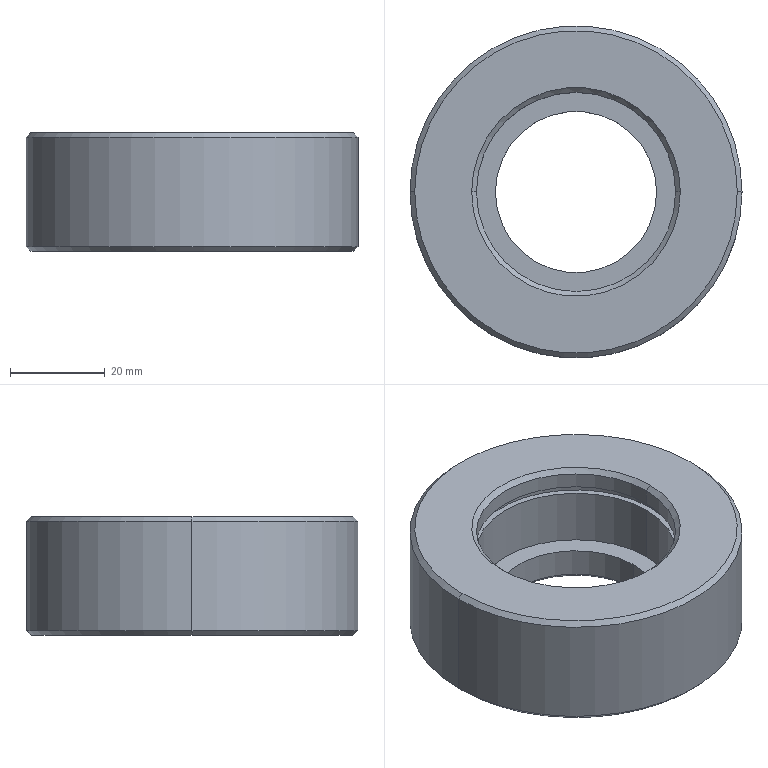Part | STEP file | 1 solid | 23 faces | box 70 x 70 x 25 mm | volume 64290 mm3 | cylinder 10 | cone 8 | plane 5 | commonest cylinder face diameters 42 x4 34 x2 44.5 x2 70 x2
STEP:
#1=CARTESIAN_POINT('',(0.,0.,0.));
#2=DIRECTION('',(0.,0.,1.));
#3=DIRECTION('',(1.,0.,0.));
#4=AXIS2_PLACEMENT_3D('',#1,#2,#3);
#5=CARTESIAN_POINT('',(21.,0.,20.7));
#6=VERTEX_POINT('',#5);
#7=CARTESIAN_POINT('',(-21.,0.,20.7));
#8=VERTEX_POINT('',#7);
#9=CARTESIAN_POINT('',(0.,0.,20.7));
#10=DIRECTION('',(0.,0.,1.));
#11=DIRECTION('',(1.,0.,0.));
#12=AXIS2_PLACEMENT_3D('',#9,#10,#11);
#13=CIRCLE('',#12,21.);
#14=CARTESIAN_POINT('',(0.,0.,20.7));
#15=DIRECTION('',(0.,0.,1.));
#16=DIRECTION('',(1.,0.,0.));
#17=AXIS2_PLACEMENT_3D('',#14,#15,#16);
#18=PLANE('',#17);
#19=CARTESIAN_POINT('',(0.,0.));
#20=DIRECTION('',(1.,0.));
#21=AXIS2_PLACEMENT_2D('',#19,#20);
#22=CIRCLE('',#21,21.);
#23=(GEOMETRIC_REPRESENTATION_CONTEXT(2)PARAMETRIC_REPRESENTATION_CONTEXT()REPRESENTATION_CONTEXT('',''));
#24=DEFINITIONAL_REPRESENTATION('',(#22),#23);
#25=PCURVE('',#18,#24);
#26=CARTESIAN_POINT('',(0.,0.,7.));
#27=DIRECTION('',(0.,0.,1.));
#28=DIRECTION('',(1.,0.,0.));
#29=AXIS2_PLACEMENT_3D('',#26,#27,#28);
#30=CYLINDRICAL_SURFACE('',#29,21.);
#31=CARTESIAN_POINT('',(0.,13.7));
#32=DIRECTION('',(1.,0.));
#33=VECTOR('',#32,1.);
#34=LINE('',#31,#33);
#35=(GEOMETRIC_REPRESENTATION_CONTEXT(2)PARAMETRIC_REPRESENTATION_CONTEXT()REPRESENTATION_CONTEXT('',''));
#36=DEFINITIONAL_REPRESENTATION('',(#34),#35);
#37=PCURVE('',#30,#36);
#38=SURFACE_CURVE('',#13,(#25,#37),.PCURVE_S1.);
#39=EDGE_CURVE('',#6,#8,#38,.T.);
#40=ORIENTED_EDGE('',*,*,#39,.T.);
#41=CARTESIAN_POINT('',(0.,0.,20.7));
#42=DIRECTION('',(0.,0.,1.));
#43=DIRECTION('',(1.,0.,0.));
#44=AXIS2_PLACEMENT_3D('',#41,#42,#43);
#45=CIRCLE('',#44,21.);
#46=CARTESIAN_POINT('',(0.,0.));
#47=DIRECTION('',(1.,0.));
#48=AXIS2_PLACEMENT_2D('',#46,#47);
#49=CIRCLE('',#48,21.);
#50=(GEOMETRIC_REPRESENTATION_CONTEXT(2)PARAMETRIC_REPRESENTATION_CONTEXT()REPRESENTATION_CONTEXT('',''));
#51=DEFINITIONAL_REPRESENTATION('',(#49),#50);
#52=PCURVE('',#18,#51);
#53=CARTESIAN_POINT('',(0.,0.,7.));
#54=DIRECTION('',(0.,0.,1.));
#55=DIRECTION('',(1.,0.,0.));
#56=AXIS2_PLACEMENT_3D('',#53,#54,#55);
#57=CYLINDRICAL_SURFACE('',#56,21.);
#58=CARTESIAN_POINT('',(0.,13.7));
#59=DIRECTION('',(1.,0.));
#60=VECTOR('',#59,1.);
#61=LINE('',#58,#60);
#62=(GEOMETRIC_REPRESENTATION_CONTEXT(2)PARAMETRIC_REPRESENTATION_CONTEXT()REPRESENTATION_CONTEXT('',''));
#63=DEFINITIONAL_REPRESENTATION('',(#61),#62);
#64=PCURVE('',#57,#63);
#65=SURFACE_CURVE('',#45,(#52,#64),.PCURVE_S1.);
#66=EDGE_CURVE('',#8,#6,#65,.T.);
#67=ORIENTED_EDGE('',*,*,#66,.T.);
#68=EDGE_LOOP('',(#40,#67));
#69=FACE_BOUND('',#68,.T.);
#70=CARTESIAN_POINT('',(-22.25,0.,20.7));
#71=VERTEX_POINT('',#70);
#72=CARTESIAN_POINT('',(22.25,0.,20.7));
#73=VERTEX_POINT('',#72);
#74=CARTESIAN_POINT('',(0.,0.,20.7));
#75=DIRECTION('',(0.,0.,-1.));
#76=DIRECTION('',(-1.,0.,0.));
#77=AXIS2_PLACEMENT_3D('',#74,#75,#76);
#78=CIRCLE('',#77,22.25);
#79=CARTESIAN_POINT('',(-22.25,0.));
#80=CARTESIAN_POINT('',(-22.25,38.538));
#81=CARTESIAN_POINT('',(11.125,19.269));
#82=CARTESIAN_POINT('',(44.5,0.));
#83=CARTESIAN_POINT('',(11.125,-19.269));
#84=CARTESIAN_POINT('',(-22.25,-38.538));
#85=CARTESIAN_POINT('',(-22.25,0.));
#86=(BOUNDED_CURVE()B_SPLINE_CURVE(2,(#79,#80,#81,#82,#83,#84,#85),.UNSPECIFIED.,.T.,.F.)B_SPLINE_CURVE_WITH_KNOTS((1,2,2,2,2,1),(-2.094,0.,2.094,4.189,6.283,8.378),.UNSPECIFIED.)CURVE()GEOMETRIC_REPRESENTATION_ITEM()RATIONAL_B_SPLINE_CURVE((1.,0.5,1.,0.5,1.,0.5,1.))REPRESENTATION_ITEM(''));
#87=(GEOMETRIC_REPRESENTATION_CONTEXT(2)PARAMETRIC_REPRESENTATION_CONTEXT()REPRESENTATION_CONTEXT('',''));
#88=DEFINITIONAL_REPRESENTATION('',(#86),#87);
#89=PCURVE('',#18,#88);
#90=CARTESIAN_POINT('',(0.,0.,20.7));
#91=DIRECTION('',(0.,0.,-1.));
#92=DIRECTION('',(-1.,0.,0.));
#93=AXIS2_PLACEMENT_3D('',#90,#91,#92);
#94=CYLINDRICAL_SURFACE('',#93,22.25);
#95=CARTESIAN_POINT('',(0.,0.));
#96=DIRECTION('',(1.,0.));
#97=VECTOR('',#96,1.);
#98=LINE('',#95,#97);
#99=(GEOMETRIC_REPRESENTATION_CONTEXT(2)PARAMETRIC_REPRESENTATION_CONTEXT()REPRESENTATION_CONTEXT('',''));
#100=DEFINITIONAL_REPRESENTATION('',(#98),#99);
#101=PCURVE('',#94,#100);
#102=SURFACE_CURVE('',#78,(#89,#101),.PCURVE_S1.);
#103=EDGE_CURVE('',#71,#73,#102,.T.);
#104=ORIENTED_EDGE('',*,*,#103,.T.);
#105=CARTESIAN_POINT('',(0.,0.,20.7));
#106=DIRECTION('',(0.,0.,-1.));
#107=DIRECTION('',(-1.,0.,0.));
#108=AXIS2_PLACEMENT_3D('',#105,#106,#107);
#109=CIRCLE('',#108,22.25);
#110=CARTESIAN_POINT('',(-22.25,0.));
#111=CARTESIAN_POINT('',(-22.25,38.538));
#112=CARTESIAN_POINT('',(11.125,19.269));
#113=CARTESIAN_POINT('',(44.5,0.));
#114=CARTESIAN_POINT('',(11.125,-19.269));
#115=CARTESIAN_POINT('',(-22.25,-38.538));
#116=CARTESIAN_POINT('',(-22.25,0.));
#117=(BOUNDED_CURVE()B_SPLINE_CURVE(2,(#110,#111,#112,#113,#114,#115,#116),.UNSPECIFIED.,.T.,.F.)B_SPLINE_CURVE_WITH_KNOTS((1,2,2,2,2,1),(-2.094,0.,2.094,4.189,6.283,8.378),.UNSPECIFIED.)CURVE()GEOMETRIC_REPRESENTATION_ITEM()RATIONAL_B_SPLINE_CURVE((1.,0.5,1.,0.5,1.,0.5,1.))REPRESENTATION_ITEM(''));
#118=(GEOMETRIC_REPRESENTATION_CONTEXT(2)PARAMETRIC_REPRESENTATION_CONTEXT()REPRESENTATION_CONTEXT('',''));
#119=DEFINITIONAL_REPRESENTATION('',(#117),#118);
#120=PCURVE('',#18,#119);
#121=CARTESIAN_POINT('',(0.,0.,20.7));
#122=DIRECTION('',(0.,0.,-1.));
#123=DIRECTION('',(-1.,0.,0.));
#124=AXIS2_PLACEMENT_3D('',#121,#122,#123);
#125=CYLINDRICAL_SURFACE('',#124,22.25);
#126=CARTESIAN_POINT('',(0.,0.));
#127=DIRECTION('',(1.,0.));
#128=VECTOR('',#127,1.);
#129=LINE('',#126,#128);
#130=(GEOMETRIC_REPRESENTATION_CONTEXT(2)PARAMETRIC_REPRESENTATION_CONTEXT()REPRESENTATION_CONTEXT('',''));
#131=DEFINITIONAL_REPRESENTATION('',(#129),#130);
#132=PCURVE('',#125,#131);
#133=SURFACE_CURVE('',#109,(#120,#132),.PCURVE_S1.);
#134=EDGE_CURVE('',#73,#71,#133,.T.);
#135=ORIENTED_EDGE('',*,*,#134,.T.);
#136=EDGE_LOOP('',(#104,#135));
#137=FACE_BOUND('',#136,.T.);
#138=ADVANCED_FACE('',(#69,#137),#18,.F.);
#139=CARTESIAN_POINT('',(21.,0.,24.));
#140=VERTEX_POINT('',#139);
#141=CARTESIAN_POINT('',(-21.,0.,24.));
#142=VERTEX_POINT('',#141);
#143=CARTESIAN_POINT('',(0.,0.,24.));
#144=DIRECTION('',(0.,0.,1.));
#145=DIRECTION('',(1.,0.,0.));
#146=AXIS2_PLACEMENT_3D('',#143,#144,#145);
#147=CIRCLE('',#146,21.);
#148=CARTESIAN_POINT('',(0.,17.));
#149=DIRECTION('',(1.,0.));
#150=VECTOR('',#149,1.);
#151=LINE('',#148,#150);
#152=(GEOMETRIC_REPRESENTATION_CONTEXT(2)PARAMETRIC_REPRESENTATION_CONTEXT()REPRESENTATION_CONTEXT('',''));
#153=DEFINITIONAL_REPRESENTATION('',(#151),#152);
#154=PCURVE('',#30,#153);
#155=CARTESIAN_POINT('',(0.,0.,25.));
#156=DIRECTION('',(0.,0.,1.));
#157=DIRECTION('',(1.,0.,0.));
#158=AXIS2_PLACEMENT_3D('',#155,#156,#157);
#159=CONICAL_SURFACE('',#158,22.,0.7854);
#160=CARTESIAN_POINT('',(0.,-1.));
#161=DIRECTION('',(1.,0.));
#162=VECTOR('',#161,1.);
#163=LINE('',#160,#162);
#164=(GEOMETRIC_REPRESENTATION_CONTEXT(2)PARAMETRIC_REPRESENTATION_CONTEXT()REPRESENTATION_CONTEXT('',''));
#165=DEFINITIONAL_REPRESENTATION('',(#163),#164);
#166=PCURVE('',#159,#165);
#167=SURFACE_CURVE('',#147,(#154,#166),.PCURVE_S1.);
#168=EDGE_CURVE('',#140,#142,#167,.T.);
#169=ORIENTED_EDGE('',*,*,#168,.F.);
#170=CARTESIAN_POINT('',(21.,0.,7.));
#171=DIRECTION('',(0.,0.,1.));
#172=VECTOR('',#171,1.);
#173=LINE('',#170,#172);
#174=CARTESIAN_POINT('',(0.,0.));
#175=DIRECTION('',(0.,1.));
#176=VECTOR('',#175,1.);
#177=LINE('',#174,#176);
#178=(GEOMETRIC_REPRESENTATION_CONTEXT(2)PARAMETRIC_REPRESENTATION_CONTEXT()REPRESENTATION_CONTEXT('',''));
#179=DEFINITIONAL_REPRESENTATION('',(#177),#178);
#180=PCURVE('',#30,#179);
#181=CARTESIAN_POINT('',(6.283,0.));
#182=DIRECTION('',(0.,1.));
#183=VECTOR('',#182,1.);
#184=LINE('',#181,#183);
#185=(GEOMETRIC_REPRESENTATION_CONTEXT(2)PARAMETRIC_REPRESENTATION_CONTEXT()REPRESENTATION_CONTEXT('',''));
#186=DEFINITIONAL_REPRESENTATION('',(#184),#185);
#187=PCURVE('',#57,#186);
#188=SURFACE_CURVE('',#173,(#180,#187),.PCURVE_S1.);
#189=EDGE_CURVE('',#6,#140,#188,.T.);
#190=ORIENTED_EDGE('',*,*,#189,.F.);
#191=ORIENTED_EDGE('',*,*,#39,.T.);
#192=CARTESIAN_POINT('',(-21.,0.,7.));
#193=DIRECTION('',(0.,0.,1.));
#194=VECTOR('',#193,1.);
#195=LINE('',#192,#194);
#196=CARTESIAN_POINT('',(3.142,0.));
#197=DIRECTION('',(0.,1.));
#198=VECTOR('',#197,1.);
#199=LINE('',#196,#198);
#200=(GEOMETRIC_REPRESENTATION_CONTEXT(2)PARAMETRIC_REPRESENTATION_CONTEXT()REPRESENTATION_CONTEXT('',''));
#201=DEFINITIONAL_REPRESENTATION('',(#199),#200);
#202=PCURVE('',#30,#201);
#203=CARTESIAN_POINT('',(3.142,0.));
#204=DIRECTION('',(0.,1.));
#205=VECTOR('',#204,1.);
#206=LINE('',#203,#205);
#207=(GEOMETRIC_REPRESENTATION_CONTEXT(2)PARAMETRIC_REPRESENTATION_CONTEXT()REPRESENTATION_CONTEXT('',''));
#208=DEFINITIONAL_REPRESENTATION('',(#206),#207);
#209=PCURVE('',#57,#208);
#210=SURFACE_CURVE('',#195,(#202,#209),.PCURVE_S1.);
#211=EDGE_CURVE('',#8,#142,#210,.T.);
#212=ORIENTED_EDGE('',*,*,#211,.T.);
#213=EDGE_LOOP('',(#169,#190,#191,#212));
#214=FACE_BOUND('',#213,.F.);
#215=ADVANCED_FACE('',(#214),#30,.F.);
#216=CARTESIAN_POINT('',(22.25,0.,19.));
#217=VERTEX_POINT('',#216);
#218=CARTESIAN_POINT('',(-22.25,0.,19.));
#219=VERTEX_POINT('',#218);
#220=CARTESIAN_POINT('',(0.,0.,19.));
#221=DIRECTION('',(0.,0.,1.));
#222=DIRECTION('',(-1.,0.,0.));
#223=AXIS2_PLACEMENT_3D('',#220,#221,#222);
#224=CIRCLE('',#223,22.25);
#225=CARTESIAN_POINT('',(6.283,1.7));
#226=DIRECTION('',(-1.,0.));
#227=VECTOR('',#226,1.);
#228=LINE('',#225,#227);
#229=(GEOMETRIC_REPRESENTATION_CONTEXT(2)PARAMETRIC_REPRESENTATION_CONTEXT()REPRESENTATION_CONTEXT('',''));
#230=DEFINITIONAL_REPRESENTATION('',(#228),#229);
#231=PCURVE('',#94,#230);
#232=CARTESIAN_POINT('',(0.,0.,19.));
#233=DIRECTION('',(0.,0.,1.));
#234=DIRECTION('',(1.,0.,0.));
#235=AXIS2_PLACEMENT_3D('',#232,#233,#234);
#236=PLANE('',#235);
#237=CARTESIAN_POINT('',(0.,0.));
#238=DIRECTION('',(-1.,0.));
#239=AXIS2_PLACEMENT_2D('',#237,#238);
#240=CIRCLE('',#239,22.25);
#241=(GEOMETRIC_REPRESENTATION_CONTEXT(2)PARAMETRIC_REPRESENTATION_CONTEXT()REPRESENTATION_CONTEXT('',''));
#242=DEFINITIONAL_REPRESENTATION('',(#240),#241);
#243=PCURVE('',#236,#242);
#244=SURFACE_CURVE('',#224,(#231,#243),.PCURVE_S1.);
#245=EDGE_CURVE('',#217,#219,#244,.T.);
#246=ORIENTED_EDGE('',*,*,#245,.T.);
#247=CARTESIAN_POINT('',(-22.25,0.,20.7));
#248=DIRECTION('',(0.,0.,-1.));
#249=VECTOR('',#248,1.);
#250=LINE('',#247,#249);
#251=CARTESIAN_POINT('',(0.,0.));
#252=DIRECTION('',(0.,1.));
#253=VECTOR('',#252,1.);
#254=LINE('',#251,#253);
#255=(GEOMETRIC_REPRESENTATION_CONTEXT(2)PARAMETRIC_REPRESENTATION_CONTEXT()REPRESENTATION_CONTEXT('',''));
#256=DEFINITIONAL_REPRESENTATION('',(#254),#255);
#257=PCURVE('',#94,#256);
#258=CARTESIAN_POINT('',(6.283,0.));
#259=DIRECTION('',(0.,1.));
#260=VECTOR('',#259,1.);
#261=LINE('',#258,#260);
#262=(GEOMETRIC_REPRESENTATION_CONTEXT(2)PARAMETRIC_REPRESENTATION_CONTEXT()REPRESENTATION_CONTEXT('',''));
#263=DEFINITIONAL_REPRESENTATION('',(#261),#262);
#264=PCURVE('',#125,#263);
#265=SURFACE_CURVE('',#250,(#257,#264),.PCURVE_S1.);
#266=EDGE_CURVE('',#71,#219,#265,.T.);
#267=ORIENTED_EDGE('',*,*,#266,.F.);
#268=ORIENTED_EDGE('',*,*,#103,.T.);
#269=CARTESIAN_POINT('',(22.25,0.,20.7));
#270=DIRECTION('',(0.,0.,-1.));
#271=VECTOR('',#270,1.);
#272=LINE('',#269,#271);
#273=CARTESIAN_POINT('',(3.142,0.));
#274=DIRECTION('',(0.,1.));
#275=VECTOR('',#274,1.);
#276=LINE('',#273,#275);
#277=(GEOMETRIC_REPRESENTATION_CONTEXT(2)PARAMETRIC_REPRESENTATION_CONTEXT()REPRESENTATION_CONTEXT('',''));
#278=DEFINITIONAL_REPRESENTATION('',(#276),#277);
#279=PCURVE('',#94,#278);
#280=CARTESIAN_POINT('',(3.142,0.));
#281=DIRECTION('',(0.,1.));
#282=VECTOR('',#281,1.);
#283=LINE('',#280,#282);
#284=(GEOMETRIC_REPRESENTATION_CONTEXT(2)PARAMETRIC_REPRESENTATION_CONTEXT()REPRESENTATION_CONTEXT('',''));
#285=DEFINITIONAL_REPRESENTATION('',(#283),#284);
#286=PCURVE('',#125,#285);
#287=SURFACE_CURVE('',#272,(#279,#286),.PCURVE_S1.);
#288=EDGE_CURVE('',#73,#217,#287,.T.);
#289=ORIENTED_EDGE('',*,*,#288,.T.);
#290=EDGE_LOOP('',(#246,#267,#268,#289));
#291=FACE_BOUND('',#290,.F.);
#292=ADVANCED_FACE('',(#291),#94,.F.);
#293=CARTESIAN_POINT('',(-22.,0.,25.));
#294=VERTEX_POINT('',#293);
#295=CARTESIAN_POINT('',(22.,0.,25.));
#296=VERTEX_POINT('',#295);
#297=CARTESIAN_POINT('',(0.,0.,25.));
#298=DIRECTION('',(0.,0.,-1.));
#299=DIRECTION('',(1.,0.,0.));
#300=AXIS2_PLACEMENT_3D('',#297,#298,#299);
#301=CIRCLE('',#300,22.);
#302=CARTESIAN_POINT('',(6.283,0.));
#303=DIRECTION('',(-1.,0.));
#304=VECTOR('',#303,1.);
#305=LINE('',#302,#304);
#306=(GEOMETRIC_REPRESENTATION_CONTEXT(2)PARAMETRIC_REPRESENTATION_CONTEXT()REPRESENTATION_CONTEXT('',''));
#307=DEFINITIONAL_REPRESENTATION('',(#305),#306);
#308=PCURVE('',#159,#307);
#309=CARTESIAN_POINT('',(0.,0.,25.));
#310=DIRECTION('',(0.,0.,1.));
#311=DIRECTION('',(1.,0.,0.));
#312=AXIS2_PLACEMENT_3D('',#309,#310,#311);
#313=PLANE('',#312);
#314=CARTESIAN_POINT('',(22.,0.));
#315=CARTESIAN_POINT('',(22.,-38.105));
#316=CARTESIAN_POINT('',(-11.,-19.053));
#317=CARTESIAN_POINT('',(-44.,0.));
#318=CARTESIAN_POINT('',(-11.,19.053));
#319=CARTESIAN_POINT('',(22.,38.105));
#320=CARTESIAN_POINT('',(22.,0.));
#321=(BOUNDED_CURVE()B_SPLINE_CURVE(2,(#314,#315,#316,#317,#318,#319,#320),.UNSPECIFIED.,.T.,.F.)B_SPLINE_CURVE_WITH_KNOTS((1,2,2,2,2,1),(-2.094,0.,2.094,4.189,6.283,8.378),.UNSPECIFIED.)CURVE()GEOMETRIC_REPRESENTATION_ITEM()RATIONAL_B_SPLINE_CURVE((1.,0.5,1.,0.5,1.,0.5,1.))REPRESENTATION_ITEM(''));
#322=(GEOMETRIC_REPRESENTATION_CONTEXT(2)PARAMETRIC_REPRESENTATION_CONTEXT()REPRESENTATION_CONTEXT('',''));
#323=DEFINITIONAL_REPRESENTATION('',(#321),#322);
#324=PCURVE('',#313,#323);
#325=SURFACE_CURVE('',#301,(#308,#324),.PCURVE_S1.);
#326=EDGE_CURVE('',#294,#296,#325,.T.);
#327=ORIENTED_EDGE('',*,*,#326,.T.);
#328=CARTESIAN_POINT('',(22.,0.,25.));
#329=DIRECTION('',(0.7071,0.,0.7071));
#330=VECTOR('',#329,1.);
#331=LINE('',#328,#330);
#332=CARTESIAN_POINT('',(0.,0.));
#333=DIRECTION('',(0.,1.));
#334=VECTOR('',#333,1.);
#335=LINE('',#332,#334);
#336=(GEOMETRIC_REPRESENTATION_CONTEXT(2)PARAMETRIC_REPRESENTATION_CONTEXT()REPRESENTATION_CONTEXT('',''));
#337=DEFINITIONAL_REPRESENTATION('',(#335),#336);
#338=PCURVE('',#159,#337);
#339=CARTESIAN_POINT('',(0.,0.,25.));
#340=DIRECTION('',(0.,0.,1.));
#341=DIRECTION('',(1.,0.,0.));
#342=AXIS2_PLACEMENT_3D('',#339,#340,#341);
#343=CONICAL_SURFACE('',#342,22.,0.7854);
#344=CARTESIAN_POINT('',(6.283,0.));
#345=DIRECTION('',(0.,1.));
#346=VECTOR('',#345,1.);
#347=LINE('',#344,#346);
#348=(GEOMETRIC_REPRESENTATION_CONTEXT(2)PARAMETRIC_REPRESENTATION_CONTEXT()REPRESENTATION_CONTEXT('',''));
#349=DEFINITIONAL_REPRESENTATION('',(#347),#348);
#350=PCURVE('',#343,#349);
#351=SURFACE_CURVE('',#331,(#338,#350),.PCURVE_S1.);
#352=EDGE_CURVE('',#140,#296,#351,.T.);
#353=ORIENTED_EDGE('',*,*,#352,.F.);
#354=ORIENTED_EDGE('',*,*,#168,.T.);
#355=CARTESIAN_POINT('',(-22.,0.,25.));
#356=DIRECTION('',(-0.7071,0.,0.7071));
#357=VECTOR('',#356,1.);
#358=LINE('',#355,#357);
#359=CARTESIAN_POINT('',(3.142,0.));
#360=DIRECTION('',(0.,1.));
#361=VECTOR('',#360,1.);
#362=LINE('',#359,#361);
#363=(GEOMETRIC_REPRESENTATION_CONTEXT(2)PARAMETRIC_REPRESENTATION_CONTEXT()REPRESENTATION_CONTEXT('',''));
#364=DEFINITIONAL_REPRESENTATION('',(#362),#363);
#365=PCURVE('',#159,#364);
#366=CARTESIAN_POINT('',(3.142,0.));
#367=DIRECTION('',(0.,1.));
#368=VECTOR('',#367,1.);
#369=LINE('',#366,#368);
#370=(GEOMETRIC_REPRESENTATION_CONTEXT(2)PARAMETRIC_REPRESENTATION_CONTEXT()REPRESENTATION_CONTEXT('',''));
#371=DEFINITIONAL_REPRESENTATION('',(#369),#370);
#372=PCURVE('',#343,#371);
#373=SURFACE_CURVE('',#358,(#365,#372),.PCURVE_S1.);
#374=EDGE_CURVE('',#142,#294,#373,.T.);
#375=ORIENTED_EDGE('',*,*,#374,.T.);
#376=EDGE_LOOP('',(#327,#353,#354,#375));
#377=FACE_BOUND('',#376,.F.);
#378=ADVANCED_FACE('',(#377),#159,.F.);
#379=CARTESIAN_POINT('',(21.,0.,19.));
#380=VERTEX_POINT('',#379);
#381=CARTESIAN_POINT('',(-21.,0.,19.));
#382=VERTEX_POINT('',#381);
#383=CARTESIAN_POINT('',(0.,0.,19.));
#384=DIRECTION('',(0.,0.,-1.));
#385=DIRECTION('',(1.,0.,0.));
#386=AXIS2_PLACEMENT_3D('',#383,#384,#385);
#387=CIRCLE('',#386,21.);
#388=CARTESIAN_POINT('',(21.,0.));
#389=CARTESIAN_POINT('',(21.,-36.373));
#390=CARTESIAN_POINT('',(-10.5,-18.187));
#391=CARTESIAN_POINT('',(-42.,0.));
#392=CARTESIAN_POINT('',(-10.5,18.187));
#393=CARTESIAN_POINT('',(21.,36.373));
#394=CARTESIAN_POINT('',(21.,0.));
#395=(BOUNDED_CURVE()B_SPLINE_CURVE(2,(#388,#389,#390,#391,#392,#393,#394),.UNSPECIFIED.,.T.,.F.)B_SPLINE_CURVE_WITH_KNOTS((1,2,2,2,2,1),(-2.094,0.,2.094,4.189,6.283,8.378),.UNSPECIFIED.)CURVE()GEOMETRIC_REPRESENTATION_ITEM()RATIONAL_B_SPLINE_CURVE((1.,0.5,1.,0.5,1.,0.5,1.))REPRESENTATION_ITEM(''));
#396=(GEOMETRIC_REPRESENTATION_CONTEXT(2)PARAMETRIC_REPRESENTATION_CONTEXT()REPRESENTATION_CONTEXT('',''));
#397=DEFINITIONAL_REPRESENTATION('',(#395),#396);
#398=PCURVE('',#236,#397);
#399=CARTESIAN_POINT('',(0.,0.,7.));
#400=DIRECTION('',(0.,0.,1.));
#401=DIRECTION('',(1.,0.,0.));
#402=AXIS2_PLACEMENT_3D('',#399,#400,#401);
#403=CYLINDRICAL_SURFACE('',#402,21.);
#404=CARTESIAN_POINT('',(6.283,12.));
#405=DIRECTION('',(-1.,0.));
#406=VECTOR('',#405,1.);
#407=LINE('',#404,#406);
#408=(GEOMETRIC_REPRESENTATION_CONTEXT(2)PARAMETRIC_REPRESENTATION_CONTEXT()REPRESENTATION_CONTEXT('',''));
#409=DEFINITIONAL_REPRESENTATION('',(#407),#408);
#410=PCURVE('',#403,#409);
#411=SURFACE_CURVE('',#387,(#398,#410),.PCURVE_S1.);
#412=EDGE_CURVE('',#380,#382,#411,.T.);
#413=ORIENTED_EDGE('',*,*,#412,.T.);
#414=CARTESIAN_POINT('',(0.,0.,19.));
#415=DIRECTION('',(0.,0.,-1.));
#416=DIRECTION('',(1.,0.,0.));
#417=AXIS2_PLACEMENT_3D('',#414,#415,#416);
#418=CIRCLE('',#417,21.);
#419=CARTESIAN_POINT('',(21.,0.));
#420=CARTESIAN_POINT('',(21.,-36.373));
#421=CARTESIAN_POINT('',(-10.5,-18.187));
#422=CARTESIAN_POINT('',(-42.,0.));
#423=CARTESIAN_POINT('',(-10.5,18.187));
#424=CARTESIAN_POINT('',(21.,36.373));
#425=CARTESIAN_POINT('',(21.,0.));
#426=(BOUNDED_CURVE()B_SPLINE_CURVE(2,(#419,#420,#421,#422,#423,#424,#425),.UNSPECIFIED.,.T.,.F.)B_SPLINE_CURVE_WITH_KNOTS((1,2,2,2,2,1),(-2.094,0.,2.094,4.189,6.283,8.378),.UNSPECIFIED.)CURVE()GEOMETRIC_REPRESENTATION_ITEM()RATIONAL_B_SPLINE_CURVE((1.,0.5,1.,0.5,1.,0.5,1.))REPRESENTATION_ITEM(''));
#427=(GEOMETRIC_REPRESENTATION_CONTEXT(2)PARAMETRIC_REPRESENTATION_CONTEXT()REPRESENTATION_CONTEXT('',''));
#428=DEFINITIONAL_REPRESENTATION('',(#426),#427);
#429=PCURVE('',#236,#428);
#430=CARTESIAN_POINT('',(0.,0.,7.));
#431=DIRECTION('',(0.,0.,1.));
#432=DIRECTION('',(1.,0.,0.));
#433=AXIS2_PLACEMENT_3D('',#430,#431,#432);
#434=CYLINDRICAL_SURFACE('',#433,21.);
#435=CARTESIAN_POINT('',(6.283,12.));
#436=DIRECTION('',(-1.,0.));
#437=VECTOR('',#436,1.);
#438=LINE('',#435,#437);
#439=(GEOMETRIC_REPRESENTATION_CONTEXT(2)PARAMETRIC_REPRESENTATION_CONTEXT()REPRESENTATION_CONTEXT('',''));
#440=DEFINITIONAL_REPRESENTATION('',(#438),#439);
#441=PCURVE('',#434,#440);
#442=SURFACE_CURVE('',#418,(#429,#441),.PCURVE_S1.);
#443=EDGE_CURVE('',#382,#380,#442,.T.);
#444=ORIENTED_EDGE('',*,*,#443,.T.);
#445=EDGE_LOOP('',(#413,#444));
#446=FACE_BOUND('',#445,.T.);
#447=CARTESIAN_POINT('',(0.,0.,19.));
#448=DIRECTION('',(0.,0.,1.));
#449=DIRECTION('',(-1.,0.,0.));
#450=AXIS2_PLACEMENT_3D('',#447,#448,#449);
#451=CIRCLE('',#450,22.25);
#452=CARTESIAN_POINT('',(0.,0.));
#453=DIRECTION('',(-1.,0.));
#454=AXIS2_PLACEMENT_2D('',#452,#453);
#455=CIRCLE('',#454,22.25);
#456=(GEOMETRIC_REPRESENTATION_CONTEXT(2)PARAMETRIC_REPRESENTATION_CONTEXT()REPRESENTATION_CONTEXT('',''));
#457=DEFINITIONAL_REPRESENTATION('',(#455),#456);
#458=PCURVE('',#236,#457);
#459=CARTESIAN_POINT('',(6.283,1.7));
#460=DIRECTION('',(-1.,0.));
#461=VECTOR('',#460,1.);
#462=LINE('',#459,#461);
#463=(GEOMETRIC_REPRESENTATION_CONTEXT(2)PARAMETRIC_REPRESENTATION_CONTEXT()REPRESENTATION_CONTEXT('',''));
#464=DEFINITIONAL_REPRESENTATION('',(#462),#463);
#465=PCURVE('',#125,#464);
#466=SURFACE_CURVE('',#451,(#458,#465),.PCURVE_S1.);
#467=EDGE_CURVE('',#219,#217,#466,.T.);
#468=ORIENTED_EDGE('',*,*,#467,.T.);
#469=ORIENTED_EDGE('',*,*,#245,.T.);
#470=EDGE_LOOP('',(#468,#469));
#471=FACE_BOUND('',#470,.T.);
#472=ADVANCED_FACE('',(#446,#471),#236,.T.);
#473=CARTESIAN_POINT('',(0.,0.,25.));
#474=DIRECTION('',(0.,0.,-1.));
#475=DIRECTION('',(1.,0.,0.));
#476=AXIS2_PLACEMENT_3D('',#473,#474,#475);
#477=CIRCLE('',#476,22.);
#478=CARTESIAN_POINT('',(22.,0.));
#479=CARTESIAN_POINT('',(22.,-38.105));
#480=CARTESIAN_POINT('',(-11.,-19.053));
#481=CARTESIAN_POINT('',(-44.,0.));
#482=CARTESIAN_POINT('',(-11.,19.053));
#483=CARTESIAN_POINT('',(22.,38.105));
#484=CARTESIAN_POINT('',(22.,0.));
#485=(BOUNDED_CURVE()B_SPLINE_CURVE(2,(#478,#479,#480,#481,#482,#483,#484),.UNSPECIFIED.,.T.,.F.)B_SPLINE_CURVE_WITH_KNOTS((1,2,2,2,2,1),(-2.094,0.,2.094,4.189,6.283,8.378),.UNSPECIFIED.)CURVE()GEOMETRIC_REPRESENTATION_ITEM()RATIONAL_B_SPLINE_CURVE((1.,0.5,1.,0.5,1.,0.5,1.))REPRESENTATION_ITEM(''));
#486=(GEOMETRIC_REPRESENTATION_CONTEXT(2)PARAMETRIC_REPRESENTATION_CONTEXT()REPRESENTATION_CONTEXT('',''));
#487=DEFINITIONAL_REPRESENTATION('',(#485),#486);
#488=PCURVE('',#313,#487);
#489=CARTESIAN_POINT('',(6.283,0.));
#490=DIRECTION('',(-1.,0.));
#491=VECTOR('',#490,1.);
#492=LINE('',#489,#491);
#493=(GEOMETRIC_REPRESENTATION_CONTEXT(2)PARAMETRIC_REPRESENTATION_CONTEXT()REPRESENTATION_CONTEXT('',''));
#494=DEFINITIONAL_REPRESENTATION('',(#492),#493);
#495=PCURVE('',#343,#494);
#496=SURFACE_CURVE('',#477,(#488,#495),.PCURVE_S1.);
#497=EDGE_CURVE('',#296,#294,#496,.T.);
#498=ORIENTED_EDGE('',*,*,#497,.T.);
#499=ORIENTED_EDGE('',*,*,#326,.T.);
#500=EDGE_LOOP('',(#498,#499));
#501=FACE_BOUND('',#500,.T.);
#502=CARTESIAN_POINT('',(-34.,0.,25.));
#503=VERTEX_POINT('',#502);
#504=CARTESIAN_POINT('',(34.,0.,25.));
#505=VERTEX_POINT('',#504);
#506=CARTESIAN_POINT('',(0.,0.,25.));
#507=DIRECTION('',(0.,0.,-1.));
#508=DIRECTION('',(-1.,0.,0.));
#509=AXIS2_PLACEMENT_3D('',#506,#507,#508);
#510=CIRCLE('',#509,34.);
#511=CARTESIAN_POINT('',(-34.,0.));
#512=CARTESIAN_POINT('',(-34.,58.89));
#513=CARTESIAN_POINT('',(17.,29.445));
#514=CARTESIAN_POINT('',(68.,0.));
#515=CARTESIAN_POINT('',(17.,-29.445));
#516=CARTESIAN_POINT('',(-34.,-58.89));
#517=CARTESIAN_POINT('',(-34.,0.));
#518=(BOUNDED_CURVE()B_SPLINE_CURVE(2,(#511,#512,#513,#514,#515,#516,#517),.UNSPECIFIED.,.T.,.F.)B_SPLINE_CURVE_WITH_KNOTS((1,2,2,2,2,1),(-2.094,0.,2.094,4.189,6.283,8.378),.UNSPECIFIED.)CURVE()GEOMETRIC_REPRESENTATION_ITEM()RATIONAL_B_SPLINE_CURVE((1.,0.5,1.,0.5,1.,0.5,1.))REPRESENTATION_ITEM(''));
#519=(GEOMETRIC_REPRESENTATION_CONTEXT(2)PARAMETRIC_REPRESENTATION_CONTEXT()REPRESENTATION_CONTEXT('',''));
#520=DEFINITIONAL_REPRESENTATION('',(#518),#519);
#521=PCURVE('',#313,#520);
#522=CARTESIAN_POINT('',(0.,0.,24.));
#523=DIRECTION('',(0.,0.,-1.));
#524=DIRECTION('',(-1.,0.,0.));
#525=AXIS2_PLACEMENT_3D('',#522,#523,#524);
#526=CONICAL_SURFACE('',#525,35.,0.7854);
#527=CARTESIAN_POINT('',(0.,-1.));
#528=DIRECTION('',(1.,0.));
#529=VECTOR('',#528,1.);
#530=LINE('',#527,#529);
#531=(GEOMETRIC_REPRESENTATION_CONTEXT(2)PARAMETRIC_REPRESENTATION_CONTEXT()REPRESENTATION_CONTEXT('',''));
#532=DEFINITIONAL_REPRESENTATION('',(#530),#531);
#533=PCURVE('',#526,#532);
#534=SURFACE_CURVE('',#510,(#521,#533),.PCURVE_S1.);
#535=EDGE_CURVE('',#503,#505,#534,.T.);
#536=ORIENTED_EDGE('',*,*,#535,.F.);
#537=CARTESIAN_POINT('',(0.,0.,25.));
#538=DIRECTION('',(0.,0.,-1.));
#539=DIRECTION('',(-1.,0.,0.));
#540=AXIS2_PLACEMENT_3D('',#537,#538,#539);
#541=CIRCLE('',#540,34.);
#542=CARTESIAN_POINT('',(-34.,0.));
#543=CARTESIAN_POINT('',(-34.,58.89));
#544=CARTESIAN_POINT('',(17.,29.445));
#545=CARTESIAN_POINT('',(68.,0.));
#546=CARTESIAN_POINT('',(17.,-29.445));
#547=CARTESIAN_POINT('',(-34.,-58.89));
#548=CARTESIAN_POINT('',(-34.,0.));
#549=(BOUNDED_CURVE()B_SPLINE_CURVE(2,(#542,#543,#544,#545,#546,#547,#548),.UNSPECIFIED.,.T.,.F.)B_SPLINE_CURVE_WITH_KNOTS((1,2,2,2,2,1),(-2.094,0.,2.094,4.189,6.283,8.378),.UNSPECIFIED.)CURVE()GEOMETRIC_REPRESENTATION_ITEM()RATIONAL_B_SPLINE_CURVE((1.,0.5,1.,0.5,1.,0.5,1.))REPRESENTATION_ITEM(''));
#550=(GEOMETRIC_REPRESENTATION_CONTEXT(2)PARAMETRIC_REPRESENTATION_CONTEXT()REPRESENTATION_CONTEXT('',''));
#551=DEFINITIONAL_REPRESENTATION('',(#549),#550);
#552=PCURVE('',#313,#551);
#553=CARTESIAN_POINT('',(0.,0.,24.));
#554=DIRECTION('',(0.,0.,-1.));
#555=DIRECTION('',(-1.,0.,0.));
#556=AXIS2_PLACEMENT_3D('',#553,#554,#555);
#557=CONICAL_SURFACE('',#556,35.,0.7854);
#558=CARTESIAN_POINT('',(0.,-1.));
#559=DIRECTION('',(1.,0.));
#560=VECTOR('',#559,1.);
#561=LINE('',#558,#560);
#562=(GEOMETRIC_REPRESENTATION_CONTEXT(2)PARAMETRIC_REPRESENTATION_CONTEXT()REPRESENTATION_CONTEXT('',''));
#563=DEFINITIONAL_REPRESENTATION('',(#561),#562);
#564=PCURVE('',#557,#563);
#565=SURFACE_CURVE('',#541,(#552,#564),.PCURVE_S1.);
#566=EDGE_CURVE('',#505,#503,#565,.T.);
#567=ORIENTED_EDGE('',*,*,#566,.F.);
#568=EDGE_LOOP('',(#536,#567));
#569=FACE_BOUND('',#568,.T.);
#570=ADVANCED_FACE('',(#501,#569),#313,.T.);
#571=ORIENTED_EDGE('',*,*,#443,.T.);
#572=CARTESIAN_POINT('',(21.,0.,7.));
#573=VERTEX_POINT('',#572);
#574=CARTESIAN_POINT('',(21.,0.,7.));
#575=DIRECTION('',(0.,0.,1.));
#576=VECTOR('',#575,1.);
#577=LINE('',#574,#576);
#578=CARTESIAN_POINT('',(0.,0.));
#579=DIRECTION('',(0.,1.));
#580=VECTOR('',#579,1.);
#581=LINE('',#578,#580);
#582=(GEOMETRIC_REPRESENTATION_CONTEXT(2)PARAMETRIC_REPRESENTATION_CONTEXT()REPRESENTATION_CONTEXT('',''));
#583=DEFINITIONAL_REPRESENTATION('',(#581),#582);
#584=PCURVE('',#434,#583);
#585=CARTESIAN_POINT('',(6.283,0.));
#586=DIRECTION('',(0.,1.));
#587=VECTOR('',#586,1.);
#588=LINE('',#585,#587);
#589=(GEOMETRIC_REPRESENTATION_CONTEXT(2)PARAMETRIC_REPRESENTATION_CONTEXT()REPRESENTATION_CONTEXT('',''));
#590=DEFINITIONAL_REPRESENTATION('',(#588),#589);
#591=PCURVE('',#403,#590);
#592=SURFACE_CURVE('',#577,(#584,#591),.PCURVE_S1.);
#593=EDGE_CURVE('',#573,#380,#592,.T.);
#594=ORIENTED_EDGE('',*,*,#593,.F.);
#595=CARTESIAN_POINT('',(-21.,0.,7.));
#596=VERTEX_POINT('',#595);
#597=CARTESIAN_POINT('',(0.,0.,7.));
#598=DIRECTION('',(0.,0.,1.));
#599=DIRECTION('',(1.,0.,0.));
#600=AXIS2_PLACEMENT_3D('',#597,#598,#599);
#601=CIRCLE('',#600,21.);
#602=CARTESIAN_POINT('',(0.,0.));
#603=DIRECTION('',(1.,0.));
#604=VECTOR('',#603,1.);
#605=LINE('',#602,#604);
#606=(GEOMETRIC_REPRESENTATION_CONTEXT(2)PARAMETRIC_REPRESENTATION_CONTEXT()REPRESENTATION_CONTEXT('',''));
#607=DEFINITIONAL_REPRESENTATION('',(#605),#606);
#608=PCURVE('',#434,#607);
#609=CARTESIAN_POINT('',(0.,0.,7.));
#610=DIRECTION('',(0.,0.,1.));
#611=DIRECTION('',(1.,0.,0.));
#612=AXIS2_PLACEMENT_3D('',#609,#610,#611);
#613=PLANE('',#612);
#614=CARTESIAN_POINT('',(0.,0.));
#615=DIRECTION('',(1.,0.));
#616=AXIS2_PLACEMENT_2D('',#614,#615);
#617=CIRCLE('',#616,21.);
#618=(GEOMETRIC_REPRESENTATION_CONTEXT(2)PARAMETRIC_REPRESENTATION_CONTEXT()REPRESENTATION_CONTEXT('',''));
#619=DEFINITIONAL_REPRESENTATION('',(#617),#618);
#620=PCURVE('',#613,#619);
#621=SURFACE_CURVE('',#601,(#608,#620),.PCURVE_S1.);
#622=EDGE_CURVE('',#573,#596,#621,.T.);
#623=ORIENTED_EDGE('',*,*,#622,.T.);
#624=CARTESIAN_POINT('',(-21.,0.,7.));
#625=DIRECTION('',(0.,0.,1.));
#626=VECTOR('',#625,1.);
#627=LINE('',#624,#626);
#628=CARTESIAN_POINT('',(3.142,0.));
#629=DIRECTION('',(0.,1.));
#630=VECTOR('',#629,1.);
#631=LINE('',#628,#630);
#632=(GEOMETRIC_REPRESENTATION_CONTEXT(2)PARAMETRIC_REPRESENTATION_CONTEXT()REPRESENTATION_CONTEXT('',''));
#633=DEFINITIONAL_REPRESENTATION('',(#631),#632);
#634=PCURVE('',#434,#633);
#635=CARTESIAN_POINT('',(3.142,0.));
#636=DIRECTION('',(0.,1.));
#637=VECTOR('',#636,1.);
#638=LINE('',#635,#637);
#639=(GEOMETRIC_REPRESENTATION_CONTEXT(2)PARAMETRIC_REPRESENTATION_CONTEXT()REPRESENTATION_CONTEXT('',''));
#640=DEFINITIONAL_REPRESENTATION('',(#638),#639);
#641=PCURVE('',#403,#640);
#642=SURFACE_CURVE('',#627,(#634,#641),.PCURVE_S1.);
#643=EDGE_CURVE('',#596,#382,#642,.T.);
#644=ORIENTED_EDGE('',*,*,#643,.T.);
#645=EDGE_LOOP('',(#571,#594,#623,#644));
#646=FACE_BOUND('',#645,.F.);
#647=ADVANCED_FACE('',(#646),#434,.F.);
#648=CARTESIAN_POINT('',(35.,0.,24.));
#649=VERTEX_POINT('',#648);
#650=CARTESIAN_POINT('',(35.,0.,24.));
#651=DIRECTION('',(0.7071,0.,-0.7071));
#652=VECTOR('',#651,1.);
#653=LINE('',#650,#652);
#654=CARTESIAN_POINT('',(3.142,0.));
#655=DIRECTION('',(0.,1.));
#656=VECTOR('',#655,1.);
#657=LINE('',#654,#656);
#658=(GEOMETRIC_REPRESENTATION_CONTEXT(2)PARAMETRIC_REPRESENTATION_CONTEXT()REPRESENTATION_CONTEXT('',''));
#659=DEFINITIONAL_REPRESENTATION('',(#657),#658);
#660=PCURVE('',#557,#659);
#661=CARTESIAN_POINT('',(3.142,0.));
#662=DIRECTION('',(0.,1.));
#663=VECTOR('',#662,1.);
#664=LINE('',#661,#663);
#665=(GEOMETRIC_REPRESENTATION_CONTEXT(2)PARAMETRIC_REPRESENTATION_CONTEXT()REPRESENTATION_CONTEXT('',''));
#666=DEFINITIONAL_REPRESENTATION('',(#664),#665);
#667=PCURVE('',#526,#666);
#668=SURFACE_CURVE('',#653,(#660,#667),.PCURVE_S1.);
#669=EDGE_CURVE('',#505,#649,#668,.T.);
#670=ORIENTED_EDGE('',*,*,#669,.F.);
#671=ORIENTED_EDGE('',*,*,#566,.T.);
#672=CARTESIAN_POINT('',(-35.,0.,24.));
#673=VERTEX_POINT('',#672);
#674=CARTESIAN_POINT('',(-35.,0.,24.));
#675=DIRECTION('',(-0.7071,0.,-0.7071));
#676=VECTOR('',#675,1.);
#677=LINE('',#674,#676);
#678=CARTESIAN_POINT('',(6.283,0.));
#679=DIRECTION('',(0.,1.));
#680=VECTOR('',#679,1.);
#681=LINE('',#678,#680);
#682=(GEOMETRIC_REPRESENTATION_CONTEXT(2)PARAMETRIC_REPRESENTATION_CONTEXT()REPRESENTATION_CONTEXT('',''));
#683=DEFINITIONAL_REPRESENTATION('',(#681),#682);
#684=PCURVE('',#557,#683);
#685=CARTESIAN_POINT('',(0.,0.));
#686=DIRECTION('',(0.,1.));
#687=VECTOR('',#686,1.);
#688=LINE('',#685,#687);
#689=(GEOMETRIC_REPRESENTATION_CONTEXT(2)PARAMETRIC_REPRESENTATION_CONTEXT()REPRESENTATION_CONTEXT('',''));
#690=DEFINITIONAL_REPRESENTATION('',(#688),#689);
#691=PCURVE('',#526,#690);
#692=SURFACE_CURVE('',#677,(#684,#691),.PCURVE_S1.);
#693=EDGE_CURVE('',#503,#673,#692,.T.);
#694=ORIENTED_EDGE('',*,*,#693,.T.);
#695=CARTESIAN_POINT('',(0.,0.,24.));
#696=DIRECTION('',(0.,0.,-1.));
#697=DIRECTION('',(-1.,0.,0.));
#698=AXIS2_PLACEMENT_3D('',#695,#696,#697);
#699=CIRCLE('',#698,35.);
#700=CARTESIAN_POINT('',(0.,0.));
#701=DIRECTION('',(1.,0.));
#702=VECTOR('',#701,1.);
#703=LINE('',#700,#702);
#704=(GEOMETRIC_REPRESENTATION_CONTEXT(2)PARAMETRIC_REPRESENTATION_CONTEXT()REPRESENTATION_CONTEXT('',''));
#705=DEFINITIONAL_REPRESENTATION('',(#703),#704);
#706=PCURVE('',#557,#705);
#707=CARTESIAN_POINT('',(0.,0.,25.));
#708=DIRECTION('',(0.,0.,-1.));
#709=DIRECTION('',(-1.,0.,0.));
#710=AXIS2_PLACEMENT_3D('',#707,#708,#709);
#711=CYLINDRICAL_SURFACE('',#710,35.);
#712=CARTESIAN_POINT('',(0.,1.));
#713=DIRECTION('',(1.,0.));
#714=VECTOR('',#713,1.);
#715=LINE('',#712,#714);
#716=(GEOMETRIC_REPRESENTATION_CONTEXT(2)PARAMETRIC_REPRESENTATION_CONTEXT()REPRESENTATION_CONTEXT('',''));
#717=DEFINITIONAL_REPRESENTATION('',(#715),#716);
#718=PCURVE('',#711,#717);
#719=SURFACE_CURVE('',#699,(#706,#718),.PCURVE_S1.);
#720=EDGE_CURVE('',#649,#673,#719,.T.);
#721=ORIENTED_EDGE('',*,*,#720,.F.);
#722=EDGE_LOOP('',(#670,#671,#694,#721));
#723=FACE_BOUND('',#722,.T.);
#724=ADVANCED_FACE('',(#723),#557,.T.);
#725=CARTESIAN_POINT('',(17.,0.,7.));
#726=VERTEX_POINT('',#725);
#727=CARTESIAN_POINT('',(-17.,0.,7.));
#728=VERTEX_POINT('',#727);
#729=CARTESIAN_POINT('',(0.,0.,7.));
#730=DIRECTION('',(0.,0.,-1.));
#731=DIRECTION('',(1.,0.,0.));
#732=AXIS2_PLACEMENT_3D('',#729,#730,#731);
#733=CIRCLE('',#732,17.);
#734=CARTESIAN_POINT('',(17.,0.));
#735=CARTESIAN_POINT('',(17.,-29.445));
#736=CARTESIAN_POINT('',(-8.5,-14.722));
#737=CARTESIAN_POINT('',(-34.,0.));
#738=CARTESIAN_POINT('',(-8.5,14.722));
#739=CARTESIAN_POINT('',(17.,29.445));
#740=CARTESIAN_POINT('',(17.,0.));
#741=(BOUNDED_CURVE()B_SPLINE_CURVE(2,(#734,#735,#736,#737,#738,#739,#740),.UNSPECIFIED.,.T.,.F.)B_SPLINE_CURVE_WITH_KNOTS((1,2,2,2,2,1),(-2.094,0.,2.094,4.189,6.283,8.378),.UNSPECIFIED.)CURVE()GEOMETRIC_REPRESENTATION_ITEM()RATIONAL_B_SPLINE_CURVE((1.,0.5,1.,0.5,1.,0.5,1.))REPRESENTATION_ITEM(''));
#742=(GEOMETRIC_REPRESENTATION_CONTEXT(2)PARAMETRIC_REPRESENTATION_CONTEXT()REPRESENTATION_CONTEXT('',''));
#743=DEFINITIONAL_REPRESENTATION('',(#741),#742);
#744=PCURVE('',#613,#743);
#745=CARTESIAN_POINT('',(0.,0.,-0.001));
#746=DIRECTION('',(0.,0.,1.));
#747=DIRECTION('',(1.,0.,0.));
#748=AXIS2_PLACEMENT_3D('',#745,#746,#747);
#749=CYLINDRICAL_SURFACE('',#748,17.);
#750=CARTESIAN_POINT('',(6.283,7.001));
#751=DIRECTION('',(-1.,0.));
#752=VECTOR('',#751,1.);
#753=LINE('',#750,#752);
#754=(GEOMETRIC_REPRESENTATION_CONTEXT(2)PARAMETRIC_REPRESENTATION_CONTEXT()REPRESENTATION_CONTEXT('',''));
#755=DEFINITIONAL_REPRESENTATION('',(#753),#754);
#756=PCURVE('',#749,#755);
#757=SURFACE_CURVE('',#733,(#744,#756),.PCURVE_S1.);
#758=EDGE_CURVE('',#726,#728,#757,.T.);
#759=ORIENTED_EDGE('',*,*,#758,.T.);
#760=CARTESIAN_POINT('',(0.,0.,7.));
#761=DIRECTION('',(0.,0.,-1.));
#762=DIRECTION('',(1.,0.,0.));
#763=AXIS2_PLACEMENT_3D('',#760,#761,#762);
#764=CIRCLE('',#763,17.);
#765=CARTESIAN_POINT('',(17.,0.));
#766=CARTESIAN_POINT('',(17.,-29.445));
#767=CARTESIAN_POINT('',(-8.5,-14.722));
#768=CARTESIAN_POINT('',(-34.,0.));
#769=CARTESIAN_POINT('',(-8.5,14.722));
#770=CARTESIAN_POINT('',(17.,29.445));
#771=CARTESIAN_POINT('',(17.,0.));
#772=(BOUNDED_CURVE()B_SPLINE_CURVE(2,(#765,#766,#767,#768,#769,#770,#771),.UNSPECIFIED.,.T.,.F.)B_SPLINE_CURVE_WITH_KNOTS((1,2,2,2,2,1),(-2.094,0.,2.094,4.189,6.283,8.378),.UNSPECIFIED.)CURVE()GEOMETRIC_REPRESENTATION_ITEM()RATIONAL_B_SPLINE_CURVE((1.,0.5,1.,0.5,1.,0.5,1.))REPRESENTATION_ITEM(''));
#773=(GEOMETRIC_REPRESENTATION_CONTEXT(2)PARAMETRIC_REPRESENTATION_CONTEXT()REPRESENTATION_CONTEXT('',''));
#774=DEFINITIONAL_REPRESENTATION('',(#772),#773);
#775=PCURVE('',#613,#774);
#776=CARTESIAN_POINT('',(0.,0.,-0.001));
#777=DIRECTION('',(0.,0.,1.));
#778=DIRECTION('',(1.,0.,0.));
#779=AXIS2_PLACEMENT_3D('',#776,#777,#778);
#780=CYLINDRICAL_SURFACE('',#779,17.);
#781=CARTESIAN_POINT('',(6.283,7.001));
#782=DIRECTION('',(-1.,0.));
#783=VECTOR('',#782,1.);
#784=LINE('',#781,#783);
#785=(GEOMETRIC_REPRESENTATION_CONTEXT(2)PARAMETRIC_REPRESENTATION_CONTEXT()REPRESENTATION_CONTEXT('',''));
#786=DEFINITIONAL_REPRESENTATION('',(#784),#785);
#787=PCURVE('',#780,#786);
#788=SURFACE_CURVE('',#764,(#775,#787),.PCURVE_S1.);
#789=EDGE_CURVE('',#728,#726,#788,.T.);
#790=ORIENTED_EDGE('',*,*,#789,.T.);
#791=EDGE_LOOP('',(#759,#790));
#792=FACE_BOUND('',#791,.T.);
#793=ORIENTED_EDGE('',*,*,#622,.T.);
#794=CARTESIAN_POINT('',(0.,0.,7.));
#795=DIRECTION('',(0.,0.,1.));
#796=DIRECTION('',(1.,0.,0.));
#797=AXIS2_PLACEMENT_3D('',#794,#795,#796);
#798=CIRCLE('',#797,21.);
#799=CARTESIAN_POINT('',(0.,0.));
#800=DIRECTION('',(1.,0.));
#801=AXIS2_PLACEMENT_2D('',#799,#800);
#802=CIRCLE('',#801,21.);
#803=(GEOMETRIC_REPRESENTATION_CONTEXT(2)PARAMETRIC_REPRESENTATION_CONTEXT()REPRESENTATION_CONTEXT('',''));
#804=DEFINITIONAL_REPRESENTATION('',(#802),#803);
#805=PCURVE('',#613,#804);
#806=CARTESIAN_POINT('',(0.,0.));
#807=DIRECTION('',(1.,0.));
#808=VECTOR('',#807,1.);
#809=LINE('',#806,#808);
#810=(GEOMETRIC_REPRESENTATION_CONTEXT(2)PARAMETRIC_REPRESENTATION_CONTEXT()REPRESENTATION_CONTEXT('',''));
#811=DEFINITIONAL_REPRESENTATION('',(#809),#810);
#812=PCURVE('',#403,#811);
#813=SURFACE_CURVE('',#798,(#805,#812),.PCURVE_S1.);
#814=EDGE_CURVE('',#596,#573,#813,.T.);
#815=ORIENTED_EDGE('',*,*,#814,.T.);
#816=EDGE_LOOP('',(#793,#815));
#817=FACE_BOUND('',#816,.T.);
#818=ADVANCED_FACE('',(#792,#817),#613,.T.);
#819=CARTESIAN_POINT('',(35.,0.,1.));
#820=VERTEX_POINT('',#819);
#821=CARTESIAN_POINT('',(35.,0.,25.));
#822=DIRECTION('',(0.,0.,-1.));
#823=VECTOR('',#822,1.);
#824=LINE('',#821,#823);
#825=CARTESIAN_POINT('',(3.142,0.));
#826=DIRECTION('',(0.,1.));
#827=VECTOR('',#826,1.);
#828=LINE('',#825,#827);
#829=(GEOMETRIC_REPRESENTATION_CONTEXT(2)PARAMETRIC_REPRESENTATION_CONTEXT()REPRESENTATION_CONTEXT('',''));
#830=DEFINITIONAL_REPRESENTATION('',(#828),#829);
#831=PCURVE('',#711,#830);
#832=CARTESIAN_POINT('',(0.,0.,25.));
#833=DIRECTION('',(0.,0.,-1.));
#834=DIRECTION('',(-1.,0.,0.));
#835=AXIS2_PLACEMENT_3D('',#832,#833,#834);
#836=CYLINDRICAL_SURFACE('',#835,35.);
#837=CARTESIAN_POINT('',(3.142,0.));
#838=DIRECTION('',(0.,1.));
#839=VECTOR('',#838,1.);
#840=LINE('',#837,#839);
#841=(GEOMETRIC_REPRESENTATION_CONTEXT(2)PARAMETRIC_REPRESENTATION_CONTEXT()REPRESENTATION_CONTEXT('',''));
#842=DEFINITIONAL_REPRESENTATION('',(#840),#841);
#843=PCURVE('',#836,#842);
#844=SURFACE_CURVE('',#824,(#831,#843),.PCURVE_S1.);
#845=EDGE_CURVE('',#649,#820,#844,.T.);
#846=ORIENTED_EDGE('',*,*,#845,.F.);
#847=ORIENTED_EDGE('',*,*,#720,.T.);
#848=CARTESIAN_POINT('',(-35.,0.,1.));
#849=VERTEX_POINT('',#848);
#850=CARTESIAN_POINT('',(-35.,0.,25.));
#851=DIRECTION('',(0.,0.,-1.));
#852=VECTOR('',#851,1.);
#853=LINE('',#850,#852);
#854=CARTESIAN_POINT('',(6.283,0.));
#855=DIRECTION('',(0.,1.));
#856=VECTOR('',#855,1.);
#857=LINE('',#854,#856);
#858=(GEOMETRIC_REPRESENTATION_CONTEXT(2)PARAMETRIC_REPRESENTATION_CONTEXT()REPRESENTATION_CONTEXT('',''));
#859=DEFINITIONAL_REPRESENTATION('',(#857),#858);
#860=PCURVE('',#711,#859);
#861=CARTESIAN_POINT('',(0.,0.));
#862=DIRECTION('',(0.,1.));
#863=VECTOR('',#862,1.);
#864=LINE('',#861,#863);
#865=(GEOMETRIC_REPRESENTATION_CONTEXT(2)PARAMETRIC_REPRESENTATION_CONTEXT()REPRESENTATION_CONTEXT('',''));
#866=DEFINITIONAL_REPRESENTATION('',(#864),#865);
#867=PCURVE('',#836,#866);
#868=SURFACE_CURVE('',#853,(#860,#867),.PCURVE_S1.);
#869=EDGE_CURVE('',#673,#849,#868,.T.);
#870=ORIENTED_EDGE('',*,*,#869,.T.);
#871=CARTESIAN_POINT('',(0.,0.,1.));
#872=DIRECTION('',(0.,0.,-1.));
#873=DIRECTION('',(1.,0.,0.));
#874=AXIS2_PLACEMENT_3D('',#871,#872,#873);
#875=CIRCLE('',#874,35.);
#876=CARTESIAN_POINT('',(3.142,24.));
#877=DIRECTION('',(1.,0.));
#878=VECTOR('',#877,1.);
#879=LINE('',#876,#878);
#880=(GEOMETRIC_REPRESENTATION_CONTEXT(2)PARAMETRIC_REPRESENTATION_CONTEXT()REPRESENTATION_CONTEXT('',''));
#881=DEFINITIONAL_REPRESENTATION('',(#879),#880);
#882=PCURVE('',#711,#881);
#883=CARTESIAN_POINT('',(0.,0.,1.));
#884=DIRECTION('',(0.,0.,1.));
#885=DIRECTION('',(1.,0.,0.));
#886=AXIS2_PLACEMENT_3D('',#883,#884,#885);
#887=CONICAL_SURFACE('',#886,35.,0.7854);
#888=CARTESIAN_POINT('',(6.283,0.));
#889=DIRECTION('',(-1.,0.));
#890=VECTOR('',#889,1.);
#891=LINE('',#888,#890);
#892=(GEOMETRIC_REPRESENTATION_CONTEXT(2)PARAMETRIC_REPRESENTATION_CONTEXT()REPRESENTATION_CONTEXT('',''));
#893=DEFINITIONAL_REPRESENTATION('',(#891),#892);
#894=PCURVE('',#887,#893);
#895=SURFACE_CURVE('',#875,(#882,#894),.PCURVE_S1.);
#896=EDGE_CURVE('',#820,#849,#895,.T.);
#897=ORIENTED_EDGE('',*,*,#896,.F.);
#898=EDGE_LOOP('',(#846,#847,#870,#897));
#899=FACE_BOUND('',#898,.T.);
#900=ADVANCED_FACE('',(#899),#711,.T.);
#901=ORIENTED_EDGE('',*,*,#789,.T.);
#902=CARTESIAN_POINT('',(17.,0.,1.));
#903=VERTEX_POINT('',#902);
#904=CARTESIAN_POINT('',(17.,0.,-0.001));
#905=DIRECTION('',(0.,0.,1.));
#906=VECTOR('',#905,1.);
#907=LINE('',#904,#906);
#908=CARTESIAN_POINT('',(0.,0.));
#909=DIRECTION('',(0.,1.));
#910=VECTOR('',#909,1.);
#911=LINE('',#908,#910);
#912=(GEOMETRIC_REPRESENTATION_CONTEXT(2)PARAMETRIC_REPRESENTATION_CONTEXT()REPRESENTATION_CONTEXT('',''));
#913=DEFINITIONAL_REPRESENTATION('',(#911),#912);
#914=PCURVE('',#780,#913);
#915=CARTESIAN_POINT('',(6.283,0.));
#916=DIRECTION('',(0.,1.));
#917=VECTOR('',#916,1.);
#918=LINE('',#915,#917);
#919=(GEOMETRIC_REPRESENTATION_CONTEXT(2)PARAMETRIC_REPRESENTATION_CONTEXT()REPRESENTATION_CONTEXT('',''));
#920=DEFINITIONAL_REPRESENTATION('',(#918),#919);
#921=PCURVE('',#749,#920);
#922=SURFACE_CURVE('',#907,(#914,#921),.PCURVE_S1.);
#923=EDGE_CURVE('',#903,#726,#922,.T.);
#924=ORIENTED_EDGE('',*,*,#923,.F.);
#925=CARTESIAN_POINT('',(-17.,0.,1.));
#926=VERTEX_POINT('',#925);
#927=CARTESIAN_POINT('',(0.,0.,1.));
#928=DIRECTION('',(0.,0.,-1.));
#929=DIRECTION('',(-1.,0.,0.));
#930=AXIS2_PLACEMENT_3D('',#927,#928,#929);
#931=CIRCLE('',#930,17.);
#932=CARTESIAN_POINT('',(3.142,1.001));
#933=DIRECTION('',(-1.,0.));
#934=VECTOR('',#933,1.);
#935=LINE('',#932,#934);
#936=(GEOMETRIC_REPRESENTATION_CONTEXT(2)PARAMETRIC_REPRESENTATION_CONTEXT()REPRESENTATION_CONTEXT('',''));
#937=DEFINITIONAL_REPRESENTATION('',(#935),#936);
#938=PCURVE('',#780,#937);
#939=CARTESIAN_POINT('',(0.,0.,0.));
#940=DIRECTION('',(0.,0.,-1.));
#941=DIRECTION('',(-1.,0.,0.));
#942=AXIS2_PLACEMENT_3D('',#939,#940,#941);
#943=CONICAL_SURFACE('',#942,18.,0.7854);
#944=CARTESIAN_POINT('',(0.,-1.));
#945=DIRECTION('',(1.,0.));
#946=VECTOR('',#945,1.);
#947=LINE('',#944,#946);
#948=(GEOMETRIC_REPRESENTATION_CONTEXT(2)PARAMETRIC_REPRESENTATION_CONTEXT()REPRESENTATION_CONTEXT('',''));
#949=DEFINITIONAL_REPRESENTATION('',(#947),#948);
#950=PCURVE('',#943,#949);
#951=SURFACE_CURVE('',#931,(#938,#950),.PCURVE_S1.);
#952=EDGE_CURVE('',#926,#903,#951,.T.);
#953=ORIENTED_EDGE('',*,*,#952,.F.);
#954=CARTESIAN_POINT('',(-17.,0.,-0.001));
#955=DIRECTION('',(0.,0.,1.));
#956=VECTOR('',#955,1.);
#957=LINE('',#954,#956);
#958=CARTESIAN_POINT('',(3.142,0.));
#959=DIRECTION('',(0.,1.));
#960=VECTOR('',#959,1.);
#961=LINE('',#958,#960);
#962=(GEOMETRIC_REPRESENTATION_CONTEXT(2)PARAMETRIC_REPRESENTATION_CONTEXT()REPRESENTATION_CONTEXT('',''));
#963=DEFINITIONAL_REPRESENTATION('',(#961),#962);
#964=PCURVE('',#780,#963);
#965=CARTESIAN_POINT('',(3.142,0.));
#966=DIRECTION('',(0.,1.));
#967=VECTOR('',#966,1.);
#968=LINE('',#965,#967);
#969=(GEOMETRIC_REPRESENTATION_CONTEXT(2)PARAMETRIC_REPRESENTATION_CONTEXT()REPRESENTATION_CONTEXT('',''));
#970=DEFINITIONAL_REPRESENTATION('',(#968),#969);
#971=PCURVE('',#749,#970);
#972=SURFACE_CURVE('',#957,(#964,#971),.PCURVE_S1.);
#973=EDGE_CURVE('',#926,#728,#972,.T.);
#974=ORIENTED_EDGE('',*,*,#973,.T.);
#975=EDGE_LOOP('',(#901,#924,#953,#974));
#976=FACE_BOUND('',#975,.F.);
#977=ADVANCED_FACE('',(#976),#780,.F.);
#978=CARTESIAN_POINT('',(-34.,0.,0.));
#979=VERTEX_POINT('',#978);
#980=CARTESIAN_POINT('',(-35.,0.,1.));
#981=DIRECTION('',(-0.7071,0.,0.7071));
#982=VECTOR('',#981,1.);
#983=LINE('',#980,#982);
#984=CARTESIAN_POINT('',(3.142,0.));
#985=DIRECTION('',(0.,1.));
#986=VECTOR('',#985,1.);
#987=LINE('',#984,#986);
#988=(GEOMETRIC_REPRESENTATION_CONTEXT(2)PARAMETRIC_REPRESENTATION_CONTEXT()REPRESENTATION_CONTEXT('',''));
#989=DEFINITIONAL_REPRESENTATION('',(#987),#988);
#990=PCURVE('',#887,#989);
#991=CARTESIAN_POINT('',(0.,0.,1.));
#992=DIRECTION('',(0.,0.,1.));
#993=DIRECTION('',(1.,0.,0.));
#994=AXIS2_PLACEMENT_3D('',#991,#992,#993);
#995=CONICAL_SURFACE('',#994,35.,0.7854);
#996=CARTESIAN_POINT('',(3.142,0.));
#997=DIRECTION('',(0.,1.));
#998=VECTOR('',#997,1.);
#999=LINE('',#996,#998);
#1000=(GEOMETRIC_REPRESENTATION_CONTEXT(2)PARAMETRIC_REPRESENTATION_CONTEXT()REPRESENTATION_CONTEXT('',''));
#1001=DEFINITIONAL_REPRESENTATION('',(#999),#1000);
#1002=PCURVE('',#995,#1001);
#1003=SURFACE_CURVE('',#983,(#990,#1002),.PCURVE_S1.);
#1004=EDGE_CURVE('',#979,#849,#1003,.T.);
#1005=ORIENTED_EDGE('',*,*,#1004,.F.);
#1006=CARTESIAN_POINT('',(34.,0.,0.));
#1007=VERTEX_POINT('',#1006);
#1008=CARTESIAN_POINT('',(0.,0.,0.));
#1009=DIRECTION('',(0.,0.,1.));
#1010=DIRECTION('',(1.,0.,0.));
#1011=AXIS2_PLACEMENT_3D('',#1008,#1009,#1010);
#1012=CIRCLE('',#1011,34.);
#1013=CARTESIAN_POINT('',(0.,-1.));
#1014=DIRECTION('',(1.,0.));
#1015=VECTOR('',#1014,1.);
#1016=LINE('',#1013,#1015);
#1017=(GEOMETRIC_REPRESENTATION_CONTEXT(2)PARAMETRIC_REPRESENTATION_CONTEXT()REPRESENTATION_CONTEXT('',''));
#1018=DEFINITIONAL_REPRESENTATION('',(#1016),#1017);
#1019=PCURVE('',#887,#1018);
#1020=CARTESIAN_POINT('',(0.,0.,0.));
#1021=DIRECTION('',(0.,0.,1.));
#1022=DIRECTION('',(1.,0.,0.));
#1023=AXIS2_PLACEMENT_3D('',#1020,#1021,#1022);
#1024=PLANE('',#1023);
#1025=CARTESIAN_POINT('',(0.,0.));
#1026=DIRECTION('',(1.,0.));
#1027=AXIS2_PLACEMENT_2D('',#1025,#1026);
#1028=CIRCLE('',#1027,34.);
#1029=(GEOMETRIC_REPRESENTATION_CONTEXT(2)PARAMETRIC_REPRESENTATION_CONTEXT()REPRESENTATION_CONTEXT('',''));
#1030=DEFINITIONAL_REPRESENTATION('',(#1028),#1029);
#1031=PCURVE('',#1024,#1030);
#1032=SURFACE_CURVE('',#1012,(#1019,#1031),.PCURVE_S1.);
#1033=EDGE_CURVE('',#979,#1007,#1032,.T.);
#1034=ORIENTED_EDGE('',*,*,#1033,.T.);
#1035=CARTESIAN_POINT('',(35.,0.,1.));
#1036=DIRECTION('',(0.7071,0.,0.7071));
#1037=VECTOR('',#1036,1.);
#1038=LINE('',#1035,#1037);
#1039=CARTESIAN_POINT('',(6.283,0.));
#1040=DIRECTION('',(0.,1.));
#1041=VECTOR('',#1040,1.);
#1042=LINE('',#1039,#1041);
#1043=(GEOMETRIC_REPRESENTATION_CONTEXT(2)PARAMETRIC_REPRESENTATION_CONTEXT()REPRESENTATION_CONTEXT('',''));
#1044=DEFINITIONAL_REPRESENTATION('',(#1042),#1043);
#1045=PCURVE('',#887,#1044);
#1046=CARTESIAN_POINT('',(0.,0.));
#1047=DIRECTION('',(0.,1.));
#1048=VECTOR('',#1047,1.);
#1049=LINE('',#1046,#1048);
#1050=(GEOMETRIC_REPRESENTATION_CONTEXT(2)PARAMETRIC_REPRESENTATION_CONTEXT()REPRESENTATION_CONTEXT('',''));
#1051=DEFINITIONAL_REPRESENTATION('',(#1049),#1050);
#1052=PCURVE('',#995,#1051);
#1053=SURFACE_CURVE('',#1038,(#1045,#1052),.PCURVE_S1.);
#1054=EDGE_CURVE('',#1007,#820,#1053,.T.);
#1055=ORIENTED_EDGE('',*,*,#1054,.T.);
#1056=ORIENTED_EDGE('',*,*,#896,.T.);
#1057=EDGE_LOOP('',(#1005,#1034,#1055,#1056));
#1058=FACE_BOUND('',#1057,.T.);
#1059=ADVANCED_FACE('',(#1058),#887,.T.);
#1060=CARTESIAN_POINT('',(-18.,0.,0.));
#1061=VERTEX_POINT('',#1060);
#1062=CARTESIAN_POINT('',(18.,0.,0.));
#1063=VERTEX_POINT('',#1062);
#1064=CARTESIAN_POINT('',(0.,0.,0.));
#1065=DIRECTION('',(0.,0.,-1.));
#1066=DIRECTION('',(-1.,0.,0.));
#1067=AXIS2_PLACEMENT_3D('',#1064,#1065,#1066);
#1068=CIRCLE('',#1067,18.);
#1069=CARTESIAN_POINT('',(0.,0.));
#1070=DIRECTION('',(1.,0.));
#1071=VECTOR('',#1070,1.);
#1072=LINE('',#1069,#1071);
#1073=(GEOMETRIC_REPRESENTATION_CONTEXT(2)PARAMETRIC_REPRESENTATION_CONTEXT()REPRESENTATION_CONTEXT('',''));
#1074=DEFINITIONAL_REPRESENTATION('',(#1072),#1073);
#1075=PCURVE('',#943,#1074);
#1076=CARTESIAN_POINT('',(-18.,0.));
#1077=CARTESIAN_POINT('',(-18.,31.177));
#1078=CARTESIAN_POINT('',(9.,15.588));
#1079=CARTESIAN_POINT('',(36.,0.));
#1080=CARTESIAN_POINT('',(9.,-15.588));
#1081=CARTESIAN_POINT('',(-18.,-31.177));
#1082=CARTESIAN_POINT('',(-18.,0.));
#1083=(BOUNDED_CURVE()B_SPLINE_CURVE(2,(#1076,#1077,#1078,#1079,#1080,#1081,#1082),.UNSPECIFIED.,.T.,.F.)B_SPLINE_CURVE_WITH_KNOTS((1,2,2,2,2,1),(-2.094,0.,2.094,4.189,6.283,8.378),.UNSPECIFIED.)CURVE()GEOMETRIC_REPRESENTATION_ITEM()RATIONAL_B_SPLINE_CURVE((1.,0.5,1.,0.5,1.,0.5,1.))REPRESENTATION_ITEM(''));
#1084=(GEOMETRIC_REPRESENTATION_CONTEXT(2)PARAMETRIC_REPRESENTATION_CONTEXT()REPRESENTATION_CONTEXT('',''));
#1085=DEFINITIONAL_REPRESENTATION('',(#1083),#1084);
#1086=PCURVE('',#1024,#1085);
#1087=SURFACE_CURVE('',#1068,(#1075,#1086),.PCURVE_S1.);
#1088=EDGE_CURVE('',#1061,#1063,#1087,.T.);
#1089=ORIENTED_EDGE('',*,*,#1088,.F.);
#1090=CARTESIAN_POINT('',(-18.,0.,0.));
#1091=DIRECTION('',(-0.7071,0.,-0.7071));
#1092=VECTOR('',#1091,1.);
#1093=LINE('',#1090,#1092);
#1094=CARTESIAN_POINT('',(0.,0.));
#1095=DIRECTION('',(0.,1.));
#1096=VECTOR('',#1095,1.);
#1097=LINE('',#1094,#1096);
#1098=(GEOMETRIC_REPRESENTATION_CONTEXT(2)PARAMETRIC_REPRESENTATION_CONTEXT()REPRESENTATION_CONTEXT('',''));
#1099=DEFINITIONAL_REPRESENTATION('',(#1097),#1098);
#1100=PCURVE('',#943,#1099);
#1101=CARTESIAN_POINT('',(0.,0.,0.));
#1102=DIRECTION('',(0.,0.,-1.));
#1103=DIRECTION('',(-1.,0.,0.));
#1104=AXIS2_PLACEMENT_3D('',#1101,#1102,#1103);
#1105=CONICAL_SURFACE('',#1104,18.,0.7854);
#1106=CARTESIAN_POINT('',(6.283,0.));
#1107=DIRECTION('',(0.,1.));
#1108=VECTOR('',#1107,1.);
#1109=LINE('',#1106,#1108);
#1110=(GEOMETRIC_REPRESENTATION_CONTEXT(2)PARAMETRIC_REPRESENTATION_CONTEXT()REPRESENTATION_CONTEXT('',''));
#1111=DEFINITIONAL_REPRESENTATION('',(#1109),#1110);
#1112=PCURVE('',#1105,#1111);
#1113=SURFACE_CURVE('',#1093,(#1100,#1112),.PCURVE_S1.);
#1114=EDGE_CURVE('',#926,#1061,#1113,.T.);
#1115=ORIENTED_EDGE('',*,*,#1114,.F.);
#1116=ORIENTED_EDGE('',*,*,#952,.T.);
#1117=CARTESIAN_POINT('',(18.,0.,0.));
#1118=DIRECTION('',(0.7071,0.,-0.7071));
#1119=VECTOR('',#1118,1.);
#1120=LINE('',#1117,#1119);
#1121=CARTESIAN_POINT('',(3.142,0.));
#1122=DIRECTION('',(0.,1.));
#1123=VECTOR('',#1122,1.);
#1124=LINE('',#1121,#1123);
#1125=(GEOMETRIC_REPRESENTATION_CONTEXT(2)PARAMETRIC_REPRESENTATION_CONTEXT()REPRESENTATION_CONTEXT('',''));
#1126=DEFINITIONAL_REPRESENTATION('',(#1124),#1125);
#1127=PCURVE('',#943,#1126);
#1128=CARTESIAN_POINT('',(3.142,0.));
#1129=DIRECTION('',(0.,1.));
#1130=VECTOR('',#1129,1.);
#1131=LINE('',#1128,#1130);
#1132=(GEOMETRIC_REPRESENTATION_CONTEXT(2)PARAMETRIC_REPRESENTATION_CONTEXT()REPRESENTATION_CONTEXT('',''));
#1133=DEFINITIONAL_REPRESENTATION('',(#1131),#1132);
#1134=PCURVE('',#1105,#1133);
#1135=SURFACE_CURVE('',#1120,(#1127,#1134),.PCURVE_S1.);
#1136=EDGE_CURVE('',#903,#1063,#1135,.T.);
#1137=ORIENTED_EDGE('',*,*,#1136,.T.);
#1138=EDGE_LOOP('',(#1089,#1115,#1116,#1137));
#1139=FACE_BOUND('',#1138,.F.);
#1140=ADVANCED_FACE('',(#1139),#943,.F.);
#1141=ORIENTED_EDGE('',*,*,#1088,.F.);
#1142=CARTESIAN_POINT('',(0.,0.,0.));
#1143=DIRECTION('',(0.,0.,-1.));
#1144=DIRECTION('',(-1.,0.,0.));
#1145=AXIS2_PLACEMENT_3D('',#1142,#1143,#1144);
#1146=CIRCLE('',#1145,18.);
#1147=CARTESIAN_POINT('',(-18.,0.));
#1148=CARTESIAN_POINT('',(-18.,31.177));
#1149=CARTESIAN_POINT('',(9.,15.588));
#1150=CARTESIAN_POINT('',(36.,0.));
#1151=CARTESIAN_POINT('',(9.,-15.588));
#1152=CARTESIAN_POINT('',(-18.,-31.177));
#1153=CARTESIAN_POINT('',(-18.,0.));
#1154=(BOUNDED_CURVE()B_SPLINE_CURVE(2,(#1147,#1148,#1149,#1150,#1151,#1152,#1153),.UNSPECIFIED.,.T.,.F.)B_SPLINE_CURVE_WITH_KNOTS((1,2,2,2,2,1),(-2.094,0.,2.094,4.189,6.283,8.378),.UNSPECIFIED.)CURVE()GEOMETRIC_REPRESENTATION_ITEM()RATIONAL_B_SPLINE_CURVE((1.,0.5,1.,0.5,1.,0.5,1.))REPRESENTATION_ITEM(''));
#1155=(GEOMETRIC_REPRESENTATION_CONTEXT(2)PARAMETRIC_REPRESENTATION_CONTEXT()REPRESENTATION_CONTEXT('',''));
#1156=DEFINITIONAL_REPRESENTATION('',(#1154),#1155);
#1157=PCURVE('',#1024,#1156);
#1158=CARTESIAN_POINT('',(0.,0.));
#1159=DIRECTION('',(1.,0.));
#1160=VECTOR('',#1159,1.);
#1161=LINE('',#1158,#1160);
#1162=(GEOMETRIC_REPRESENTATION_CONTEXT(2)PARAMETRIC_REPRESENTATION_CONTEXT()REPRESENTATION_CONTEXT('',''));
#1163=DEFINITIONAL_REPRESENTATION('',(#1161),#1162);
#1164=PCURVE('',#1105,#1163);
#1165=SURFACE_CURVE('',#1146,(#1157,#1164),.PCURVE_S1.);
#1166=EDGE_CURVE('',#1063,#1061,#1165,.T.);
#1167=ORIENTED_EDGE('',*,*,#1166,.F.);
#1168=EDGE_LOOP('',(#1141,#1167));
#1169=FACE_BOUND('',#1168,.T.);
#1170=CARTESIAN_POINT('',(0.,0.,0.));
#1171=DIRECTION('',(0.,0.,1.));
#1172=DIRECTION('',(1.,0.,0.));
#1173=AXIS2_PLACEMENT_3D('',#1170,#1171,#1172);
#1174=CIRCLE('',#1173,34.);
#1175=CARTESIAN_POINT('',(0.,0.));
#1176=DIRECTION('',(1.,0.));
#1177=AXIS2_PLACEMENT_2D('',#1175,#1176);
#1178=CIRCLE('',#1177,34.);
#1179=(GEOMETRIC_REPRESENTATION_CONTEXT(2)PARAMETRIC_REPRESENTATION_CONTEXT()REPRESENTATION_CONTEXT('',''));
#1180=DEFINITIONAL_REPRESENTATION('',(#1178),#1179);
#1181=PCURVE('',#1024,#1180);
#1182=CARTESIAN_POINT('',(0.,-1.));
#1183=DIRECTION('',(1.,0.));
#1184=VECTOR('',#1183,1.);
#1185=LINE('',#1182,#1184);
#1186=(GEOMETRIC_REPRESENTATION_CONTEXT(2)PARAMETRIC_REPRESENTATION_CONTEXT()REPRESENTATION_CONTEXT('',''));
#1187=DEFINITIONAL_REPRESENTATION('',(#1185),#1186);
#1188=PCURVE('',#995,#1187);
#1189=SURFACE_CURVE('',#1174,(#1181,#1188),.PCURVE_S1.);
#1190=EDGE_CURVE('',#1007,#979,#1189,.T.);
#1191=ORIENTED_EDGE('',*,*,#1190,.F.);
#1192=ORIENTED_EDGE('',*,*,#1033,.F.);
#1193=EDGE_LOOP('',(#1191,#1192));
#1194=FACE_BOUND('',#1193,.T.);
#1195=ADVANCED_FACE('',(#1169,#1194),#1024,.F.);
#1196=ORIENTED_EDGE('',*,*,#189,.T.);
#1197=CARTESIAN_POINT('',(0.,0.,24.));
#1198=DIRECTION('',(0.,0.,1.));
#1199=DIRECTION('',(1.,0.,0.));
#1200=AXIS2_PLACEMENT_3D('',#1197,#1198,#1199);
#1201=CIRCLE('',#1200,21.);
#1202=CARTESIAN_POINT('',(0.,17.));
#1203=DIRECTION('',(1.,0.));
#1204=VECTOR('',#1203,1.);
#1205=LINE('',#1202,#1204);
#1206=(GEOMETRIC_REPRESENTATION_CONTEXT(2)PARAMETRIC_REPRESENTATION_CONTEXT()REPRESENTATION_CONTEXT('',''));
#1207=DEFINITIONAL_REPRESENTATION('',(#1205),#1206);
#1208=PCURVE('',#57,#1207);
#1209=CARTESIAN_POINT('',(0.,-1.));
#1210=DIRECTION('',(1.,0.));
#1211=VECTOR('',#1210,1.);
#1212=LINE('',#1209,#1211);
#1213=(GEOMETRIC_REPRESENTATION_CONTEXT(2)PARAMETRIC_REPRESENTATION_CONTEXT()REPRESENTATION_CONTEXT('',''));
#1214=DEFINITIONAL_REPRESENTATION('',(#1212),#1213);
#1215=PCURVE('',#343,#1214);
#1216=SURFACE_CURVE('',#1201,(#1208,#1215),.PCURVE_S1.);
#1217=EDGE_CURVE('',#142,#140,#1216,.T.);
#1218=ORIENTED_EDGE('',*,*,#1217,.F.);
#1219=ORIENTED_EDGE('',*,*,#211,.F.);
#1220=ORIENTED_EDGE('',*,*,#66,.T.);
#1221=EDGE_LOOP('',(#1196,#1218,#1219,#1220));
#1222=FACE_BOUND('',#1221,.F.);
#1223=ADVANCED_FACE('',(#1222),#57,.F.);
#1224=ORIENTED_EDGE('',*,*,#266,.T.);
#1225=ORIENTED_EDGE('',*,*,#467,.T.);
#1226=ORIENTED_EDGE('',*,*,#288,.F.);
#1227=ORIENTED_EDGE('',*,*,#134,.T.);
#1228=EDGE_LOOP('',(#1224,#1225,#1226,#1227));
#1229=FACE_BOUND('',#1228,.F.);
#1230=ADVANCED_FACE('',(#1229),#125,.F.);
#1231=ORIENTED_EDGE('',*,*,#352,.T.);
#1232=ORIENTED_EDGE('',*,*,#497,.T.);
#1233=ORIENTED_EDGE('',*,*,#374,.F.);
#1234=ORIENTED_EDGE('',*,*,#1217,.T.);
#1235=EDGE_LOOP('',(#1231,#1232,#1233,#1234));
#1236=FACE_BOUND('',#1235,.F.);
#1237=ADVANCED_FACE('',(#1236),#343,.F.);
#1238=ORIENTED_EDGE('',*,*,#593,.T.);
#1239=ORIENTED_EDGE('',*,*,#412,.T.);
#1240=ORIENTED_EDGE('',*,*,#643,.F.);
#1241=ORIENTED_EDGE('',*,*,#814,.T.);
#1242=EDGE_LOOP('',(#1238,#1239,#1240,#1241));
#1243=FACE_BOUND('',#1242,.F.);
#1244=ADVANCED_FACE('',(#1243),#403,.F.);
#1245=ORIENTED_EDGE('',*,*,#535,.T.);
#1246=ORIENTED_EDGE('',*,*,#669,.T.);
#1247=CARTESIAN_POINT('',(0.,0.,24.));
#1248=DIRECTION('',(0.,0.,-1.));
#1249=DIRECTION('',(-1.,0.,0.));
#1250=AXIS2_PLACEMENT_3D('',#1247,#1248,#1249);
#1251=CIRCLE('',#1250,35.);
#1252=CARTESIAN_POINT('',(0.,0.));
#1253=DIRECTION('',(1.,0.));
#1254=VECTOR('',#1253,1.);
#1255=LINE('',#1252,#1254);
#1256=(GEOMETRIC_REPRESENTATION_CONTEXT(2)PARAMETRIC_REPRESENTATION_CONTEXT()REPRESENTATION_CONTEXT('',''));
#1257=DEFINITIONAL_REPRESENTATION('',(#1255),#1256);
#1258=PCURVE('',#526,#1257);
#1259=CARTESIAN_POINT('',(0.,1.));
#1260=DIRECTION('',(1.,0.));
#1261=VECTOR('',#1260,1.);
#1262=LINE('',#1259,#1261);
#1263=(GEOMETRIC_REPRESENTATION_CONTEXT(2)PARAMETRIC_REPRESENTATION_CONTEXT()REPRESENTATION_CONTEXT('',''));
#1264=DEFINITIONAL_REPRESENTATION('',(#1262),#1263);
#1265=PCURVE('',#836,#1264);
#1266=SURFACE_CURVE('',#1251,(#1258,#1265),.PCURVE_S1.);
#1267=EDGE_CURVE('',#673,#649,#1266,.T.);
#1268=ORIENTED_EDGE('',*,*,#1267,.F.);
#1269=ORIENTED_EDGE('',*,*,#693,.F.);
#1270=EDGE_LOOP('',(#1245,#1246,#1268,#1269));
#1271=FACE_BOUND('',#1270,.T.);
#1272=ADVANCED_FACE('',(#1271),#526,.T.);
#1273=ORIENTED_EDGE('',*,*,#1267,.T.);
#1274=ORIENTED_EDGE('',*,*,#845,.T.);
#1275=CARTESIAN_POINT('',(0.,0.,1.));
#1276=DIRECTION('',(0.,0.,-1.));
#1277=DIRECTION('',(1.,0.,0.));
#1278=AXIS2_PLACEMENT_3D('',#1275,#1276,#1277);
#1279=CIRCLE('',#1278,35.);
#1280=CARTESIAN_POINT('',(-3.142,24.));
#1281=DIRECTION('',(1.,0.));
#1282=VECTOR('',#1281,1.);
#1283=LINE('',#1280,#1282);
#1284=(GEOMETRIC_REPRESENTATION_CONTEXT(2)PARAMETRIC_REPRESENTATION_CONTEXT()REPRESENTATION_CONTEXT('',''));
#1285=DEFINITIONAL_REPRESENTATION('',(#1283),#1284);
#1286=PCURVE('',#836,#1285);
#1287=CARTESIAN_POINT('',(6.283,0.));
#1288=DIRECTION('',(-1.,0.));
#1289=VECTOR('',#1288,1.);
#1290=LINE('',#1287,#1289);
#1291=(GEOMETRIC_REPRESENTATION_CONTEXT(2)PARAMETRIC_REPRESENTATION_CONTEXT()REPRESENTATION_CONTEXT('',''));
#1292=DEFINITIONAL_REPRESENTATION('',(#1290),#1291);
#1293=PCURVE('',#995,#1292);
#1294=SURFACE_CURVE('',#1279,(#1286,#1293),.PCURVE_S1.);
#1295=EDGE_CURVE('',#849,#820,#1294,.T.);
#1296=ORIENTED_EDGE('',*,*,#1295,.F.);
#1297=ORIENTED_EDGE('',*,*,#869,.F.);
#1298=EDGE_LOOP('',(#1273,#1274,#1296,#1297));
#1299=FACE_BOUND('',#1298,.T.);
#1300=ADVANCED_FACE('',(#1299),#836,.T.);
#1301=ORIENTED_EDGE('',*,*,#923,.T.);
#1302=ORIENTED_EDGE('',*,*,#758,.T.);
#1303=ORIENTED_EDGE('',*,*,#973,.F.);
#1304=CARTESIAN_POINT('',(0.,0.,1.));
#1305=DIRECTION('',(0.,0.,-1.));
#1306=DIRECTION('',(-1.,0.,0.));
#1307=AXIS2_PLACEMENT_3D('',#1304,#1305,#1306);
#1308=CIRCLE('',#1307,17.);
#1309=CARTESIAN_POINT('',(9.425,1.001));
#1310=DIRECTION('',(-1.,0.));
#1311=VECTOR('',#1310,1.);
#1312=LINE('',#1309,#1311);
#1313=(GEOMETRIC_REPRESENTATION_CONTEXT(2)PARAMETRIC_REPRESENTATION_CONTEXT()REPRESENTATION_CONTEXT('',''));
#1314=DEFINITIONAL_REPRESENTATION('',(#1312),#1313);
#1315=PCURVE('',#749,#1314);
#1316=CARTESIAN_POINT('',(0.,-1.));
#1317=DIRECTION('',(1.,0.));
#1318=VECTOR('',#1317,1.);
#1319=LINE('',#1316,#1318);
#1320=(GEOMETRIC_REPRESENTATION_CONTEXT(2)PARAMETRIC_REPRESENTATION_CONTEXT()REPRESENTATION_CONTEXT('',''));
#1321=DEFINITIONAL_REPRESENTATION('',(#1319),#1320);
#1322=PCURVE('',#1105,#1321);
#1323=SURFACE_CURVE('',#1308,(#1315,#1322),.PCURVE_S1.);
#1324=EDGE_CURVE('',#903,#926,#1323,.T.);
#1325=ORIENTED_EDGE('',*,*,#1324,.F.);
#1326=EDGE_LOOP('',(#1301,#1302,#1303,#1325));
#1327=FACE_BOUND('',#1326,.F.);
#1328=ADVANCED_FACE('',(#1327),#749,.F.);
#1329=ORIENTED_EDGE('',*,*,#1190,.T.);
#1330=ORIENTED_EDGE('',*,*,#1004,.T.);
#1331=ORIENTED_EDGE('',*,*,#1295,.T.);
#1332=ORIENTED_EDGE('',*,*,#1054,.F.);
#1333=EDGE_LOOP('',(#1329,#1330,#1331,#1332));
#1334=FACE_BOUND('',#1333,.T.);
#1335=ADVANCED_FACE('',(#1334),#995,.T.);
#1336=ORIENTED_EDGE('',*,*,#1114,.T.);
#1337=ORIENTED_EDGE('',*,*,#1166,.F.);
#1338=ORIENTED_EDGE('',*,*,#1136,.F.);
#1339=ORIENTED_EDGE('',*,*,#1324,.T.);
#1340=EDGE_LOOP('',(#1336,#1337,#1338,#1339));
#1341=FACE_BOUND('',#1340,.F.);
#1342=ADVANCED_FACE('',(#1341),#1105,.F.);
#1343=CLOSED_SHELL('',(#138,#215,#292,#378,#472,#570,#647,#724,#818,#900,#977,#1059,#1140,#1195,#1223,#1230,#1237,#1244,#1272,#1300,#1328,#1335,#1342));
#1344=MANIFOLD_SOLID_BREP('',#1343);
#1345=(LENGTH_UNIT()NAMED_UNIT(*)SI_UNIT(.MILLI.,.METRE.));
#1346=UNCERTAINTY_MEASURE_WITH_UNIT(LENGTH_MEASURE(0.0000001),#1345,'','');
#1347=(NAMED_UNIT(*)PLANE_ANGLE_UNIT()SI_UNIT($,.RADIAN.));
#1348=(NAMED_UNIT(*)SI_UNIT($,.STERADIAN.)SOLID_ANGLE_UNIT());
#1349=(GEOMETRIC_REPRESENTATION_CONTEXT(3)GLOBAL_UNCERTAINTY_ASSIGNED_CONTEXT((#1346))GLOBAL_UNIT_ASSIGNED_CONTEXT((#1345,#1347,#1348))REPRESENTATION_CONTEXT('',''));
#1350=ADVANCED_BREP_SHAPE_REPRESENTATION('',(#4,#1344),#1349);